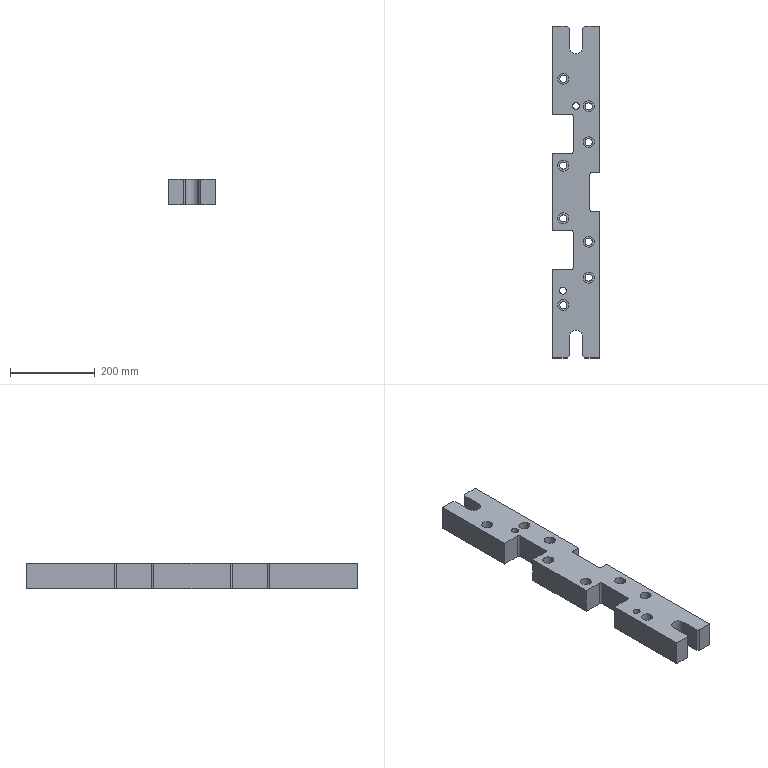Part | STEP file | PN_0008_id1770_x_t | 1 solid | 78 faces | box 110 x 785 x 60 mm | volume 3912002 mm3 | plane 46 | cylinder 32 | commonest cylinder face diameters 17 x8 26 x8 10 x6 20 x4 16 x2 16.5 x2